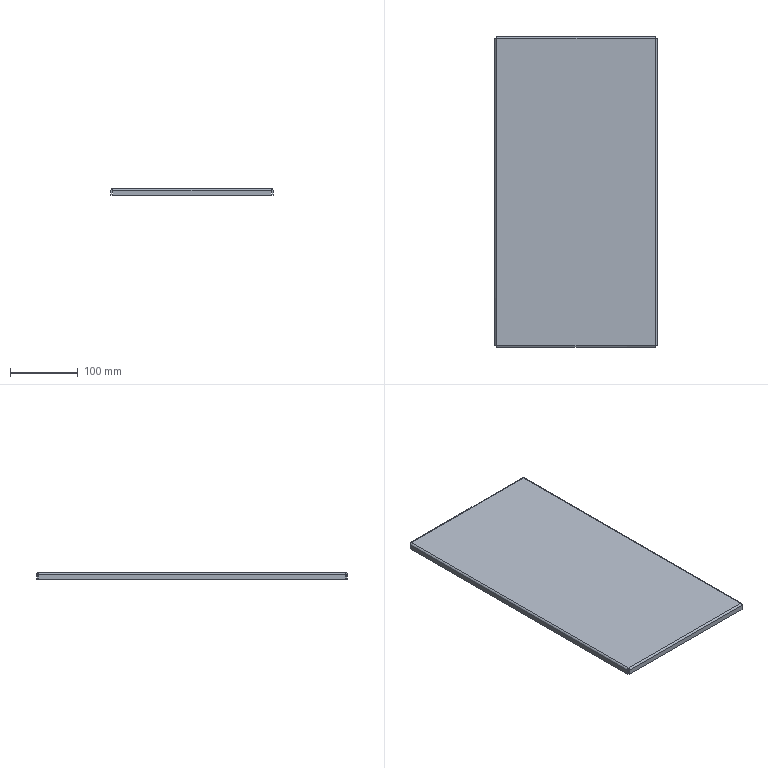Part | STEP file | 11-FG-JX01311 | 1 solid | 38 faces | box 240 x 460 x 10 mm | volume 240740 mm3 | plane 22 | spline 8 | cylinder 8 | commonest cylinder face diameters 1.473 x4 5.473 x4
STEP:
#1=CARTESIAN_POINT('',(117.263,-227.263,-2.));
#2=VERTEX_POINT('',#1);
#3=CARTESIAN_POINT('',(117.263,227.263,-2.));
#4=VERTEX_POINT('',#3);
#5=CARTESIAN_POINT('',(117.263,-227.293,-2.));
#6=DIRECTION('',(0.,1.,0.));
#7=VECTOR('',#6,1000.);
#8=LINE('',#5,#7);
#9=EDGE_CURVE('',#2,#4,#8,.T.);
#10=ORIENTED_EDGE('',*,*,#9,.F.);
#11=CARTESIAN_POINT('',(-117.263,-227.263,-2.));
#12=VERTEX_POINT('',#11);
#13=CARTESIAN_POINT('',(-117.293,-227.263,-2.));
#14=DIRECTION('',(1.,0.,0.));
#15=VECTOR('',#14,1000.);
#16=LINE('',#13,#15);
#17=EDGE_CURVE('',#12,#2,#16,.T.);
#18=ORIENTED_EDGE('',*,*,#17,.F.);
#19=CARTESIAN_POINT('',(-117.263,227.263,-2.));
#20=VERTEX_POINT('',#19);
#21=CARTESIAN_POINT('',(-117.263,227.293,-2.));
#22=DIRECTION('',(0.,-1.,0.));
#23=VECTOR('',#22,1000.);
#24=LINE('',#21,#23);
#25=EDGE_CURVE('',#20,#12,#24,.T.);
#26=ORIENTED_EDGE('',*,*,#25,.F.);
#27=CARTESIAN_POINT('',(117.293,227.263,-2.));
#28=DIRECTION('',(-1.,0.,0.));
#29=VECTOR('',#28,1000.);
#30=LINE('',#27,#29);
#31=EDGE_CURVE('',#4,#20,#30,.T.);
#32=ORIENTED_EDGE('',*,*,#31,.F.);
#33=EDGE_LOOP('',(#10,#18,#26,#32));
#34=FACE_OUTER_BOUND('',#33,.T.);
#35=CARTESIAN_POINT('',(0.,0.,-2.));
#36=DIRECTION('',(0.,0.,1.));
#37=DIRECTION('',(1.,0.,0.));
#38=AXIS2_PLACEMENT_3D('',#35,#36,#37);
#39=PLANE('',#38);
#40=ADVANCED_FACE('',(#34),#39,.F.);
#41=CARTESIAN_POINT('',(-117.263,-227.263,0.));
#42=VERTEX_POINT('',#41);
#43=CARTESIAN_POINT('',(117.263,-227.263,0.));
#44=VERTEX_POINT('',#43);
#45=CARTESIAN_POINT('',(-117.293,-227.263,0.));
#46=DIRECTION('',(1.,0.,0.));
#47=VECTOR('',#46,1000.);
#48=LINE('',#45,#47);
#49=EDGE_CURVE('',#42,#44,#48,.T.);
#50=ORIENTED_EDGE('',*,*,#49,.T.);
#51=CARTESIAN_POINT('',(117.263,227.263,0.));
#52=VERTEX_POINT('',#51);
#53=CARTESIAN_POINT('',(117.263,-227.293,0.));
#54=DIRECTION('',(0.,1.,0.));
#55=VECTOR('',#54,1000.);
#56=LINE('',#53,#55);
#57=EDGE_CURVE('',#44,#52,#56,.T.);
#58=ORIENTED_EDGE('',*,*,#57,.T.);
#59=CARTESIAN_POINT('',(-117.263,227.263,0.));
#60=VERTEX_POINT('',#59);
#61=CARTESIAN_POINT('',(117.293,227.263,0.));
#62=DIRECTION('',(-1.,0.,0.));
#63=VECTOR('',#62,1000.);
#64=LINE('',#61,#63);
#65=EDGE_CURVE('',#52,#60,#64,.T.);
#66=ORIENTED_EDGE('',*,*,#65,.T.);
#67=CARTESIAN_POINT('',(-117.263,227.293,0.));
#68=DIRECTION('',(0.,-1.,0.));
#69=VECTOR('',#68,1000.);
#70=LINE('',#67,#69);
#71=EDGE_CURVE('',#60,#42,#70,.T.);
#72=ORIENTED_EDGE('',*,*,#71,.T.);
#73=EDGE_LOOP('',(#50,#58,#66,#72));
#74=FACE_OUTER_BOUND('',#73,.T.);
#75=CARTESIAN_POINT('',(0.,0.,0.));
#76=DIRECTION('',(0.,0.,1.));
#77=DIRECTION('',(1.,0.,0.));
#78=AXIS2_PLACEMENT_3D('',#75,#76,#77);
#79=PLANE('',#78);
#80=ADVANCED_FACE('',(#74),#79,.T.);
#81=CARTESIAN_POINT('',(-117.293,230.,-2.737));
#82=VERTEX_POINT('',#81);
#83=CARTESIAN_POINT('',(-117.293,228.,-2.737));
#84=VERTEX_POINT('',#83);
#85=CARTESIAN_POINT('',(-117.293,228.,-2.737));
#86=DIRECTION('',(0.,-1.,0.));
#87=VECTOR('',#86,1000.);
#88=LINE('',#85,#87);
#89=EDGE_CURVE('',#82,#84,#88,.T.);
#90=ORIENTED_EDGE('',*,*,#89,.T.);
#91=CARTESIAN_POINT('',(-117.263,227.263,-2.));
#92=CARTESIAN_POINT('',(-117.268,227.456,-2.));
#93=CARTESIAN_POINT('',(-117.273,227.648,-2.079));
#94=CARTESIAN_POINT('',(-117.283,227.921,-2.352));
#95=CARTESIAN_POINT('',(-117.288,228.,-2.544));
#96=CARTESIAN_POINT('',(-117.293,228.,-2.737));
#97=B_SPLINE_CURVE_WITH_KNOTS('',3,(#91,#92,#93,#94,#95,#96),.UNSPECIFIED.,.F.,.F.,(4,2,4),(0.,0.5,1.),.UNSPECIFIED.);
#98=EDGE_CURVE('',#20,#84,#97,.T.);
#99=ORIENTED_EDGE('',*,*,#98,.F.);
#100=CARTESIAN_POINT('',(-117.263,227.263,-2.));
#101=DIRECTION('',(0.,0.,1.));
#102=VECTOR('',#101,1000.);
#103=LINE('',#100,#102);
#104=EDGE_CURVE('',#20,#60,#103,.T.);
#105=ORIENTED_EDGE('',*,*,#104,.T.);
#106=CARTESIAN_POINT('',(-117.263,227.263,0.));
#107=CARTESIAN_POINT('',(-117.266,227.622,0.));
#108=CARTESIAN_POINT('',(-117.268,227.98,-0.07123));
#109=CARTESIAN_POINT('',(-117.273,228.642,-0.3454));
#110=CARTESIAN_POINT('',(-117.276,228.945,-0.5482));
#111=CARTESIAN_POINT('',(-117.281,229.452,-1.055));
#112=CARTESIAN_POINT('',(-117.283,229.655,-1.358));
#113=CARTESIAN_POINT('',(-117.288,229.929,-2.02));
#114=CARTESIAN_POINT('',(-117.29,230.,-2.378));
#115=CARTESIAN_POINT('',(-117.293,230.,-2.737));
#116=B_SPLINE_CURVE_WITH_KNOTS('',3,(#106,#107,#108,#109,#110,#111,#112,#113,#114,#115),.UNSPECIFIED.,.F.,.F.,(4,2,2,2,4),(0.,0.25,0.5,0.75,1.),.UNSPECIFIED.);
#117=EDGE_CURVE('',#60,#82,#116,.T.);
#118=ORIENTED_EDGE('',*,*,#117,.T.);
#119=EDGE_LOOP('',(#90,#99,#105,#118));
#120=FACE_OUTER_BOUND('',#119,.T.);
#121=CARTESIAN_POINT('',(-117.263,227.263,0.02));
#122=CARTESIAN_POINT('',(-117.266,227.624,0.02));
#123=CARTESIAN_POINT('',(-117.268,227.985,-0.05175));
#124=CARTESIAN_POINT('',(-117.273,228.652,-0.3279));
#125=CARTESIAN_POINT('',(-117.276,228.957,-0.5322));
#126=CARTESIAN_POINT('',(-117.281,229.468,-1.043));
#127=CARTESIAN_POINT('',(-117.283,229.672,-1.348));
#128=CARTESIAN_POINT('',(-117.288,229.948,-2.015));
#129=CARTESIAN_POINT('',(-117.29,230.02,-2.376));
#130=CARTESIAN_POINT('',(-117.293,230.02,-2.737));
#131=CARTESIAN_POINT('',(-117.263,227.263,0.));
#132=CARTESIAN_POINT('',(-117.266,227.622,0.));
#133=CARTESIAN_POINT('',(-117.268,227.98,-0.07123));
#134=CARTESIAN_POINT('',(-117.273,228.642,-0.3454));
#135=CARTESIAN_POINT('',(-117.276,228.945,-0.5482));
#136=CARTESIAN_POINT('',(-117.281,229.452,-1.055));
#137=CARTESIAN_POINT('',(-117.283,229.655,-1.358));
#138=CARTESIAN_POINT('',(-117.288,229.929,-2.02));
#139=CARTESIAN_POINT('',(-117.29,230.,-2.378));
#140=CARTESIAN_POINT('',(-117.293,230.,-2.737));
#141=CARTESIAN_POINT('',(-117.263,227.263,-2.));
#142=CARTESIAN_POINT('',(-117.266,227.36,-2.));
#143=CARTESIAN_POINT('',(-117.268,227.456,-2.019));
#144=CARTESIAN_POINT('',(-117.273,227.634,-2.093));
#145=CARTESIAN_POINT('',(-117.276,227.716,-2.148));
#146=CARTESIAN_POINT('',(-117.281,227.852,-2.284));
#147=CARTESIAN_POINT('',(-117.283,227.907,-2.366));
#148=CARTESIAN_POINT('',(-117.288,227.981,-2.544));
#149=CARTESIAN_POINT('',(-117.29,228.,-2.64));
#150=CARTESIAN_POINT('',(-117.293,228.,-2.737));
#151=CARTESIAN_POINT('',(-117.263,227.263,-2.02));
#152=CARTESIAN_POINT('',(-117.266,227.357,-2.02));
#153=CARTESIAN_POINT('',(-117.268,227.451,-2.039));
#154=CARTESIAN_POINT('',(-117.273,227.624,-2.111));
#155=CARTESIAN_POINT('',(-117.276,227.704,-2.164));
#156=CARTESIAN_POINT('',(-117.281,227.836,-2.296));
#157=CARTESIAN_POINT('',(-117.283,227.889,-2.376));
#158=CARTESIAN_POINT('',(-117.288,227.961,-2.549));
#159=CARTESIAN_POINT('',(-117.29,227.98,-2.643));
#160=CARTESIAN_POINT('',(-117.293,227.98,-2.737));
#161=B_SPLINE_SURFACE_WITH_KNOTS('',1,3,((#121,#122,#123,#124,#125,#126,#127,#128,#129,#130),(#131,#132,#133,#134,#135,#136,#137,#138,#139,#140),(#141,#142,#143,#144,#145,#146,#147,#148,#149,#150),(#151,#152,#153,#154,#155,#156,#157,#158,#159,#160)),.UNSPECIFIED.,.F.,.F.,.F.,(2,1,1,2),(4,2,2,2,4),(-0.01,0.,1.,1.01),(0.,0.25,0.5,0.75,1.),.UNSPECIFIED.);
#162=ADVANCED_FACE('',(#120),#161,.F.);
#163=CARTESIAN_POINT('',(117.293,228.,-2.737));
#164=VERTEX_POINT('',#163);
#165=CARTESIAN_POINT('',(117.293,228.,-2.737));
#166=CARTESIAN_POINT('',(117.288,228.,-2.544));
#167=CARTESIAN_POINT('',(117.283,227.921,-2.352));
#168=CARTESIAN_POINT('',(117.273,227.648,-2.079));
#169=CARTESIAN_POINT('',(117.268,227.456,-2.));
#170=CARTESIAN_POINT('',(117.263,227.263,-2.));
#171=B_SPLINE_CURVE_WITH_KNOTS('',3,(#165,#166,#167,#168,#169,#170),.UNSPECIFIED.,.F.,.F.,(4,2,4),(0.,0.5,1.),.UNSPECIFIED.);
#172=EDGE_CURVE('',#164,#4,#171,.T.);
#173=ORIENTED_EDGE('',*,*,#172,.F.);
#174=CARTESIAN_POINT('',(117.293,230.,-2.737));
#175=VERTEX_POINT('',#174);
#176=CARTESIAN_POINT('',(117.293,228.,-2.737));
#177=DIRECTION('',(0.,-1.,0.));
#178=VECTOR('',#177,1000.);
#179=LINE('',#176,#178);
#180=EDGE_CURVE('',#175,#164,#179,.T.);
#181=ORIENTED_EDGE('',*,*,#180,.F.);
#182=CARTESIAN_POINT('',(117.293,230.,-2.737));
#183=CARTESIAN_POINT('',(117.29,230.,-2.378));
#184=CARTESIAN_POINT('',(117.288,229.929,-2.02));
#185=CARTESIAN_POINT('',(117.283,229.655,-1.358));
#186=CARTESIAN_POINT('',(117.281,229.452,-1.055));
#187=CARTESIAN_POINT('',(117.276,228.945,-0.5482));
#188=CARTESIAN_POINT('',(117.273,228.642,-0.3454));
#189=CARTESIAN_POINT('',(117.268,227.98,-0.07123));
#190=CARTESIAN_POINT('',(117.266,227.622,0.));
#191=CARTESIAN_POINT('',(117.263,227.263,0.));
#192=B_SPLINE_CURVE_WITH_KNOTS('',3,(#182,#183,#184,#185,#186,#187,#188,#189,#190,#191),.UNSPECIFIED.,.F.,.F.,(4,2,2,2,4),(0.,0.25,0.5,0.75,1.),.UNSPECIFIED.);
#193=EDGE_CURVE('',#175,#52,#192,.T.);
#194=ORIENTED_EDGE('',*,*,#193,.T.);
#195=CARTESIAN_POINT('',(117.263,227.263,-2.));
#196=DIRECTION('',(0.,0.,1.));
#197=VECTOR('',#196,1000.);
#198=LINE('',#195,#197);
#199=EDGE_CURVE('',#4,#52,#198,.T.);
#200=ORIENTED_EDGE('',*,*,#199,.F.);
#201=EDGE_LOOP('',(#173,#181,#194,#200));
#202=FACE_OUTER_BOUND('',#201,.T.);
#203=CARTESIAN_POINT('',(117.293,230.02,-2.737));
#204=CARTESIAN_POINT('',(117.29,230.02,-2.376));
#205=CARTESIAN_POINT('',(117.288,229.948,-2.015));
#206=CARTESIAN_POINT('',(117.283,229.672,-1.348));
#207=CARTESIAN_POINT('',(117.281,229.468,-1.043));
#208=CARTESIAN_POINT('',(117.276,228.957,-0.5322));
#209=CARTESIAN_POINT('',(117.273,228.652,-0.3279));
#210=CARTESIAN_POINT('',(117.268,227.985,-0.05175));
#211=CARTESIAN_POINT('',(117.266,227.624,0.02));
#212=CARTESIAN_POINT('',(117.263,227.263,0.02));
#213=CARTESIAN_POINT('',(117.293,230.,-2.737));
#214=CARTESIAN_POINT('',(117.29,230.,-2.378));
#215=CARTESIAN_POINT('',(117.288,229.929,-2.02));
#216=CARTESIAN_POINT('',(117.283,229.655,-1.358));
#217=CARTESIAN_POINT('',(117.281,229.452,-1.055));
#218=CARTESIAN_POINT('',(117.276,228.945,-0.5482));
#219=CARTESIAN_POINT('',(117.273,228.642,-0.3454));
#220=CARTESIAN_POINT('',(117.268,227.98,-0.07123));
#221=CARTESIAN_POINT('',(117.266,227.622,0.));
#222=CARTESIAN_POINT('',(117.263,227.263,0.));
#223=CARTESIAN_POINT('',(117.293,228.,-2.737));
#224=CARTESIAN_POINT('',(117.29,228.,-2.64));
#225=CARTESIAN_POINT('',(117.288,227.981,-2.544));
#226=CARTESIAN_POINT('',(117.283,227.907,-2.366));
#227=CARTESIAN_POINT('',(117.281,227.852,-2.284));
#228=CARTESIAN_POINT('',(117.276,227.716,-2.148));
#229=CARTESIAN_POINT('',(117.273,227.634,-2.093));
#230=CARTESIAN_POINT('',(117.268,227.456,-2.019));
#231=CARTESIAN_POINT('',(117.266,227.36,-2.));
#232=CARTESIAN_POINT('',(117.263,227.263,-2.));
#233=CARTESIAN_POINT('',(117.293,227.98,-2.737));
#234=CARTESIAN_POINT('',(117.29,227.98,-2.643));
#235=CARTESIAN_POINT('',(117.288,227.961,-2.549));
#236=CARTESIAN_POINT('',(117.283,227.889,-2.376));
#237=CARTESIAN_POINT('',(117.281,227.836,-2.296));
#238=CARTESIAN_POINT('',(117.276,227.704,-2.164));
#239=CARTESIAN_POINT('',(117.273,227.624,-2.111));
#240=CARTESIAN_POINT('',(117.268,227.451,-2.039));
#241=CARTESIAN_POINT('',(117.266,227.357,-2.02));
#242=CARTESIAN_POINT('',(117.263,227.263,-2.02));
#243=B_SPLINE_SURFACE_WITH_KNOTS('',1,3,((#203,#204,#205,#206,#207,#208,#209,#210,#211,#212),(#213,#214,#215,#216,#217,#218,#219,#220,#221,#222),(#223,#224,#225,#226,#227,#228,#229,#230,#231,#232),(#233,#234,#235,#236,#237,#238,#239,#240,#241,#242)),.UNSPECIFIED.,.F.,.F.,.F.,(2,1,1,2),(4,2,2,2,4),(-0.01,0.,1.,1.01),(0.,0.25,0.5,0.75,1.),.UNSPECIFIED.);
#244=ADVANCED_FACE('',(#202),#243,.F.);
#245=ORIENTED_EDGE('',*,*,#65,.F.);
#246=ORIENTED_EDGE('',*,*,#193,.F.);
#247=CARTESIAN_POINT('',(0.,230.,-2.737));
#248=DIRECTION('',(1.,0.,0.));
#249=VECTOR('',#248,1000.);
#250=LINE('',#247,#249);
#251=EDGE_CURVE('',#82,#175,#250,.T.);
#252=ORIENTED_EDGE('',*,*,#251,.F.);
#253=ORIENTED_EDGE('',*,*,#117,.F.);
#254=EDGE_LOOP('',(#245,#246,#252,#253));
#255=FACE_OUTER_BOUND('',#254,.T.);
#256=CARTESIAN_POINT('',(117.293,227.263,-2.737));
#257=DIRECTION('',(1.,0.,0.));
#258=DIRECTION('',(0.,1.,0.));
#259=AXIS2_PLACEMENT_3D('',#256,#257,#258);
#260=CYLINDRICAL_SURFACE('',#259,2.737);
#261=ADVANCED_FACE('',(#255),#260,.T.);
#262=ORIENTED_EDGE('',*,*,#31,.T.);
#263=ORIENTED_EDGE('',*,*,#98,.T.);
#264=CARTESIAN_POINT('',(-120.,228.,-2.737));
#265=DIRECTION('',(1.,0.,0.));
#266=VECTOR('',#265,1000.);
#267=LINE('',#264,#266);
#268=EDGE_CURVE('',#84,#164,#267,.T.);
#269=ORIENTED_EDGE('',*,*,#268,.T.);
#270=ORIENTED_EDGE('',*,*,#172,.T.);
#271=EDGE_LOOP('',(#262,#263,#269,#270));
#272=FACE_OUTER_BOUND('',#271,.T.);
#273=CARTESIAN_POINT('',(117.293,227.263,-2.737));
#274=DIRECTION('',(1.,0.,0.));
#275=DIRECTION('',(0.,1.,0.));
#276=AXIS2_PLACEMENT_3D('',#273,#274,#275);
#277=CYLINDRICAL_SURFACE('',#276,0.7366);
#278=ADVANCED_FACE('',(#272),#277,.F.);
#279=CARTESIAN_POINT('',(-117.293,228.,-10.));
#280=VERTEX_POINT('',#279);
#281=CARTESIAN_POINT('',(-117.293,230.,-10.));
#282=VERTEX_POINT('',#281);
#283=CARTESIAN_POINT('',(-117.293,230.,-10.));
#284=DIRECTION('',(0.,1.,0.));
#285=VECTOR('',#284,1000.);
#286=LINE('',#283,#285);
#287=EDGE_CURVE('',#280,#282,#286,.T.);
#288=ORIENTED_EDGE('',*,*,#287,.F.);
#289=CARTESIAN_POINT('',(-117.293,228.,0.));
#290=DIRECTION('',(0.,0.,-1.));
#291=VECTOR('',#290,1000.);
#292=LINE('',#289,#291);
#293=EDGE_CURVE('',#84,#280,#292,.T.);
#294=ORIENTED_EDGE('',*,*,#293,.F.);
#295=ORIENTED_EDGE('',*,*,#89,.F.);
#296=CARTESIAN_POINT('',(-117.293,230.,0.));
#297=DIRECTION('',(0.,0.,1.));
#298=VECTOR('',#297,1000.);
#299=LINE('',#296,#298);
#300=EDGE_CURVE('',#282,#82,#299,.T.);
#301=ORIENTED_EDGE('',*,*,#300,.F.);
#302=EDGE_LOOP('',(#288,#294,#295,#301));
#303=FACE_OUTER_BOUND('',#302,.T.);
#304=CARTESIAN_POINT('',(-117.293,228.,-2.));
#305=DIRECTION('',(-1.,0.,0.));
#306=DIRECTION('',(0.,0.,1.));
#307=AXIS2_PLACEMENT_3D('',#304,#305,#306);
#308=PLANE('',#307);
#309=ADVANCED_FACE('',(#303),#308,.T.);
#310=CARTESIAN_POINT('',(117.293,230.,-10.));
#311=VERTEX_POINT('',#310);
#312=CARTESIAN_POINT('',(117.293,230.,-2.));
#313=DIRECTION('',(0.,0.,1.));
#314=VECTOR('',#313,1000.);
#315=LINE('',#312,#314);
#316=EDGE_CURVE('',#311,#175,#315,.T.);
#317=ORIENTED_EDGE('',*,*,#316,.F.);
#318=CARTESIAN_POINT('',(120.,230.,-10.));
#319=DIRECTION('',(1.,0.,0.));
#320=VECTOR('',#319,1000.);
#321=LINE('',#318,#320);
#322=EDGE_CURVE('',#282,#311,#321,.T.);
#323=ORIENTED_EDGE('',*,*,#322,.F.);
#324=ORIENTED_EDGE('',*,*,#300,.T.);
#325=ORIENTED_EDGE('',*,*,#251,.T.);
#326=EDGE_LOOP('',(#317,#323,#324,#325));
#327=FACE_OUTER_BOUND('',#326,.T.);
#328=CARTESIAN_POINT('',(0.,230.,0.));
#329=DIRECTION('',(0.,1.,0.));
#330=DIRECTION('',(0.,0.,1.));
#331=AXIS2_PLACEMENT_3D('',#328,#329,#330);
#332=PLANE('',#331);
#333=ADVANCED_FACE('',(#327),#332,.T.);
#334=CARTESIAN_POINT('',(117.293,228.,-10.));
#335=VERTEX_POINT('',#334);
#336=CARTESIAN_POINT('',(0.,228.,-10.));
#337=DIRECTION('',(1.,0.,0.));
#338=VECTOR('',#337,1000.);
#339=LINE('',#336,#338);
#340=EDGE_CURVE('',#280,#335,#339,.T.);
#341=ORIENTED_EDGE('',*,*,#340,.T.);
#342=CARTESIAN_POINT('',(117.293,228.,-2.));
#343=DIRECTION('',(0.,0.,-1.));
#344=VECTOR('',#343,1000.);
#345=LINE('',#342,#344);
#346=EDGE_CURVE('',#164,#335,#345,.T.);
#347=ORIENTED_EDGE('',*,*,#346,.F.);
#348=ORIENTED_EDGE('',*,*,#268,.F.);
#349=ORIENTED_EDGE('',*,*,#293,.T.);
#350=EDGE_LOOP('',(#341,#347,#348,#349));
#351=FACE_OUTER_BOUND('',#350,.T.);
#352=CARTESIAN_POINT('',(0.,228.,0.));
#353=DIRECTION('',(0.,1.,0.));
#354=DIRECTION('',(0.,0.,1.));
#355=AXIS2_PLACEMENT_3D('',#352,#353,#354);
#356=PLANE('',#355);
#357=ADVANCED_FACE('',(#351),#356,.F.);
#358=CARTESIAN_POINT('',(117.293,228.,-10.));
#359=DIRECTION('',(0.,1.,0.));
#360=VECTOR('',#359,1000.);
#361=LINE('',#358,#360);
#362=EDGE_CURVE('',#335,#311,#361,.T.);
#363=ORIENTED_EDGE('',*,*,#362,.F.);
#364=ORIENTED_EDGE('',*,*,#340,.F.);
#365=ORIENTED_EDGE('',*,*,#287,.T.);
#366=ORIENTED_EDGE('',*,*,#322,.T.);
#367=EDGE_LOOP('',(#363,#364,#365,#366));
#368=FACE_OUTER_BOUND('',#367,.T.);
#369=CARTESIAN_POINT('',(120.,230.,-10.));
#370=DIRECTION('',(0.,0.,-1.));
#371=DIRECTION('',(0.,1.,0.));
#372=AXIS2_PLACEMENT_3D('',#369,#370,#371);
#373=PLANE('',#372);
#374=ADVANCED_FACE('',(#368),#373,.T.);
#375=ORIENTED_EDGE('',*,*,#346,.T.);
#376=ORIENTED_EDGE('',*,*,#362,.T.);
#377=ORIENTED_EDGE('',*,*,#316,.T.);
#378=ORIENTED_EDGE('',*,*,#180,.T.);
#379=EDGE_LOOP('',(#375,#376,#377,#378));
#380=FACE_OUTER_BOUND('',#379,.T.);
#381=CARTESIAN_POINT('',(117.293,228.,-2.));
#382=DIRECTION('',(-1.,0.,0.));
#383=DIRECTION('',(0.,0.,1.));
#384=AXIS2_PLACEMENT_3D('',#381,#382,#383);
#385=PLANE('',#384);
#386=ADVANCED_FACE('',(#380),#385,.F.);
#387=CARTESIAN_POINT('',(-120.,-227.293,-2.737));
#388=VERTEX_POINT('',#387);
#389=CARTESIAN_POINT('',(-118.,-227.293,-2.737));
#390=VERTEX_POINT('',#389);
#391=CARTESIAN_POINT('',(-118.,-227.293,-2.737));
#392=DIRECTION('',(1.,0.,0.));
#393=VECTOR('',#392,1000.);
#394=LINE('',#391,#393);
#395=EDGE_CURVE('',#388,#390,#394,.T.);
#396=ORIENTED_EDGE('',*,*,#395,.T.);
#397=CARTESIAN_POINT('',(-117.263,-227.263,-2.));
#398=CARTESIAN_POINT('',(-117.456,-227.268,-2.));
#399=CARTESIAN_POINT('',(-117.648,-227.273,-2.079));
#400=CARTESIAN_POINT('',(-117.921,-227.283,-2.352));
#401=CARTESIAN_POINT('',(-118.,-227.288,-2.544));
#402=CARTESIAN_POINT('',(-118.,-227.293,-2.737));
#403=B_SPLINE_CURVE_WITH_KNOTS('',3,(#397,#398,#399,#400,#401,#402),.UNSPECIFIED.,.F.,.F.,(4,2,4),(0.,0.5,1.),.UNSPECIFIED.);
#404=EDGE_CURVE('',#12,#390,#403,.T.);
#405=ORIENTED_EDGE('',*,*,#404,.F.);
#406=CARTESIAN_POINT('',(-117.263,-227.263,-2.));
#407=DIRECTION('',(0.,0.,1.));
#408=VECTOR('',#407,1000.);
#409=LINE('',#406,#408);
#410=EDGE_CURVE('',#12,#42,#409,.T.);
#411=ORIENTED_EDGE('',*,*,#410,.T.);
#412=CARTESIAN_POINT('',(-117.263,-227.263,0.));
#413=CARTESIAN_POINT('',(-117.622,-227.266,0.));
#414=CARTESIAN_POINT('',(-117.98,-227.268,-0.07123));
#415=CARTESIAN_POINT('',(-118.642,-227.273,-0.3454));
#416=CARTESIAN_POINT('',(-118.945,-227.276,-0.5482));
#417=CARTESIAN_POINT('',(-119.452,-227.281,-1.055));
#418=CARTESIAN_POINT('',(-119.655,-227.283,-1.358));
#419=CARTESIAN_POINT('',(-119.929,-227.288,-2.02));
#420=CARTESIAN_POINT('',(-120.,-227.29,-2.378));
#421=CARTESIAN_POINT('',(-120.,-227.293,-2.737));
#422=B_SPLINE_CURVE_WITH_KNOTS('',3,(#412,#413,#414,#415,#416,#417,#418,#419,#420,#421),.UNSPECIFIED.,.F.,.F.,(4,2,2,2,4),(0.,0.25,0.5,0.75,1.),.UNSPECIFIED.);
#423=EDGE_CURVE('',#42,#388,#422,.T.);
#424=ORIENTED_EDGE('',*,*,#423,.T.);
#425=EDGE_LOOP('',(#396,#405,#411,#424));
#426=FACE_OUTER_BOUND('',#425,.T.);
#427=CARTESIAN_POINT('',(-117.263,-227.263,0.02));
#428=CARTESIAN_POINT('',(-117.624,-227.266,0.02));
#429=CARTESIAN_POINT('',(-117.985,-227.268,-0.05175));
#430=CARTESIAN_POINT('',(-118.652,-227.273,-0.3279));
#431=CARTESIAN_POINT('',(-118.957,-227.276,-0.5322));
#432=CARTESIAN_POINT('',(-119.468,-227.281,-1.043));
#433=CARTESIAN_POINT('',(-119.672,-227.283,-1.348));
#434=CARTESIAN_POINT('',(-119.948,-227.288,-2.015));
#435=CARTESIAN_POINT('',(-120.02,-227.29,-2.376));
#436=CARTESIAN_POINT('',(-120.02,-227.293,-2.737));
#437=CARTESIAN_POINT('',(-117.263,-227.263,0.));
#438=CARTESIAN_POINT('',(-117.622,-227.266,0.));
#439=CARTESIAN_POINT('',(-117.98,-227.268,-0.07123));
#440=CARTESIAN_POINT('',(-118.642,-227.273,-0.3454));
#441=CARTESIAN_POINT('',(-118.945,-227.276,-0.5482));
#442=CARTESIAN_POINT('',(-119.452,-227.281,-1.055));
#443=CARTESIAN_POINT('',(-119.655,-227.283,-1.358));
#444=CARTESIAN_POINT('',(-119.929,-227.288,-2.02));
#445=CARTESIAN_POINT('',(-120.,-227.29,-2.378));
#446=CARTESIAN_POINT('',(-120.,-227.293,-2.737));
#447=CARTESIAN_POINT('',(-117.263,-227.263,-2.));
#448=CARTESIAN_POINT('',(-117.36,-227.266,-2.));
#449=CARTESIAN_POINT('',(-117.456,-227.268,-2.019));
#450=CARTESIAN_POINT('',(-117.634,-227.273,-2.093));
#451=CARTESIAN_POINT('',(-117.716,-227.276,-2.148));
#452=CARTESIAN_POINT('',(-117.852,-227.281,-2.284));
#453=CARTESIAN_POINT('',(-117.907,-227.283,-2.366));
#454=CARTESIAN_POINT('',(-117.981,-227.288,-2.544));
#455=CARTESIAN_POINT('',(-118.,-227.29,-2.64));
#456=CARTESIAN_POINT('',(-118.,-227.293,-2.737));
#457=CARTESIAN_POINT('',(-117.263,-227.263,-2.02));
#458=CARTESIAN_POINT('',(-117.357,-227.266,-2.02));
#459=CARTESIAN_POINT('',(-117.451,-227.268,-2.039));
#460=CARTESIAN_POINT('',(-117.624,-227.273,-2.111));
#461=CARTESIAN_POINT('',(-117.704,-227.276,-2.164));
#462=CARTESIAN_POINT('',(-117.836,-227.281,-2.296));
#463=CARTESIAN_POINT('',(-117.889,-227.283,-2.376));
#464=CARTESIAN_POINT('',(-117.961,-227.288,-2.549));
#465=CARTESIAN_POINT('',(-117.98,-227.29,-2.643));
#466=CARTESIAN_POINT('',(-117.98,-227.293,-2.737));
#467=B_SPLINE_SURFACE_WITH_KNOTS('',1,3,((#427,#428,#429,#430,#431,#432,#433,#434,#435,#436),(#437,#438,#439,#440,#441,#442,#443,#444,#445,#446),(#447,#448,#449,#450,#451,#452,#453,#454,#455,#456),(#457,#458,#459,#460,#461,#462,#463,#464,#465,#466)),.UNSPECIFIED.,.F.,.F.,.F.,(2,1,1,2),(4,2,2,2,4),(-0.01,0.,1.,1.01),(0.,0.25,0.5,0.75,1.),.UNSPECIFIED.);
#468=ADVANCED_FACE('',(#426),#467,.F.);
#469=CARTESIAN_POINT('',(-118.,227.293,-2.737));
#470=VERTEX_POINT('',#469);
#471=CARTESIAN_POINT('',(-118.,227.293,-2.737));
#472=CARTESIAN_POINT('',(-118.,227.288,-2.544));
#473=CARTESIAN_POINT('',(-117.921,227.283,-2.352));
#474=CARTESIAN_POINT('',(-117.648,227.273,-2.079));
#475=CARTESIAN_POINT('',(-117.456,227.268,-2.));
#476=CARTESIAN_POINT('',(-117.263,227.263,-2.));
#477=B_SPLINE_CURVE_WITH_KNOTS('',3,(#471,#472,#473,#474,#475,#476),.UNSPECIFIED.,.F.,.F.,(4,2,4),(0.,0.5,1.),.UNSPECIFIED.);
#478=EDGE_CURVE('',#470,#20,#477,.T.);
#479=ORIENTED_EDGE('',*,*,#478,.F.);
#480=CARTESIAN_POINT('',(-120.,227.293,-2.737));
#481=VERTEX_POINT('',#480);
#482=CARTESIAN_POINT('',(-118.,227.293,-2.737));
#483=DIRECTION('',(1.,0.,0.));
#484=VECTOR('',#483,1000.);
#485=LINE('',#482,#484);
#486=EDGE_CURVE('',#481,#470,#485,.T.);
#487=ORIENTED_EDGE('',*,*,#486,.F.);
#488=CARTESIAN_POINT('',(-120.,227.293,-2.737));
#489=CARTESIAN_POINT('',(-120.,227.29,-2.378));
#490=CARTESIAN_POINT('',(-119.929,227.288,-2.02));
#491=CARTESIAN_POINT('',(-119.655,227.283,-1.358));
#492=CARTESIAN_POINT('',(-119.452,227.281,-1.055));
#493=CARTESIAN_POINT('',(-118.945,227.276,-0.5482));
#494=CARTESIAN_POINT('',(-118.642,227.273,-0.3454));
#495=CARTESIAN_POINT('',(-117.98,227.268,-0.07123));
#496=CARTESIAN_POINT('',(-117.622,227.266,0.));
#497=CARTESIAN_POINT('',(-117.263,227.263,0.));
#498=B_SPLINE_CURVE_WITH_KNOTS('',3,(#488,#489,#490,#491,#492,#493,#494,#495,#496,#497),.UNSPECIFIED.,.F.,.F.,(4,2,2,2,4),(0.,0.25,0.5,0.75,1.),.UNSPECIFIED.);
#499=EDGE_CURVE('',#481,#60,#498,.T.);
#500=ORIENTED_EDGE('',*,*,#499,.T.);
#501=ORIENTED_EDGE('',*,*,#104,.F.);
#502=EDGE_LOOP('',(#479,#487,#500,#501));
#503=FACE_OUTER_BOUND('',#502,.T.);
#504=CARTESIAN_POINT('',(-120.02,227.293,-2.737));
#505=CARTESIAN_POINT('',(-120.02,227.29,-2.376));
#506=CARTESIAN_POINT('',(-119.948,227.288,-2.015));
#507=CARTESIAN_POINT('',(-119.672,227.283,-1.348));
#508=CARTESIAN_POINT('',(-119.468,227.281,-1.043));
#509=CARTESIAN_POINT('',(-118.957,227.276,-0.5322));
#510=CARTESIAN_POINT('',(-118.652,227.273,-0.3279));
#511=CARTESIAN_POINT('',(-117.985,227.268,-0.05175));
#512=CARTESIAN_POINT('',(-117.624,227.266,0.02));
#513=CARTESIAN_POINT('',(-117.263,227.263,0.02));
#514=CARTESIAN_POINT('',(-120.,227.293,-2.737));
#515=CARTESIAN_POINT('',(-120.,227.29,-2.378));
#516=CARTESIAN_POINT('',(-119.929,227.288,-2.02));
#517=CARTESIAN_POINT('',(-119.655,227.283,-1.358));
#518=CARTESIAN_POINT('',(-119.452,227.281,-1.055));
#519=CARTESIAN_POINT('',(-118.945,227.276,-0.5482));
#520=CARTESIAN_POINT('',(-118.642,227.273,-0.3454));
#521=CARTESIAN_POINT('',(-117.98,227.268,-0.07123));
#522=CARTESIAN_POINT('',(-117.622,227.266,0.));
#523=CARTESIAN_POINT('',(-117.263,227.263,0.));
#524=CARTESIAN_POINT('',(-118.,227.293,-2.737));
#525=CARTESIAN_POINT('',(-118.,227.29,-2.64));
#526=CARTESIAN_POINT('',(-117.981,227.288,-2.544));
#527=CARTESIAN_POINT('',(-117.907,227.283,-2.366));
#528=CARTESIAN_POINT('',(-117.852,227.281,-2.284));
#529=CARTESIAN_POINT('',(-117.716,227.276,-2.148));
#530=CARTESIAN_POINT('',(-117.634,227.273,-2.093));
#531=CARTESIAN_POINT('',(-117.456,227.268,-2.019));
#532=CARTESIAN_POINT('',(-117.36,227.266,-2.));
#533=CARTESIAN_POINT('',(-117.263,227.263,-2.));
#534=CARTESIAN_POINT('',(-117.98,227.293,-2.737));
#535=CARTESIAN_POINT('',(-117.98,227.29,-2.643));
#536=CARTESIAN_POINT('',(-117.961,227.288,-2.549));
#537=CARTESIAN_POINT('',(-117.889,227.283,-2.376));
#538=CARTESIAN_POINT('',(-117.836,227.281,-2.296));
#539=CARTESIAN_POINT('',(-117.704,227.276,-2.164));
#540=CARTESIAN_POINT('',(-117.624,227.273,-2.111));
#541=CARTESIAN_POINT('',(-117.451,227.268,-2.039));
#542=CARTESIAN_POINT('',(-117.357,227.266,-2.02));
#543=CARTESIAN_POINT('',(-117.263,227.263,-2.02));
#544=B_SPLINE_SURFACE_WITH_KNOTS('',1,3,((#504,#505,#506,#507,#508,#509,#510,#511,#512,#513),(#514,#515,#516,#517,#518,#519,#520,#521,#522,#523),(#524,#525,#526,#527,#528,#529,#530,#531,#532,#533),(#534,#535,#536,#537,#538,#539,#540,#541,#542,#543)),.UNSPECIFIED.,.F.,.F.,.F.,(2,1,1,2),(4,2,2,2,4),(-0.01,0.,1.,1.01),(0.,0.25,0.5,0.75,1.),.UNSPECIFIED.);
#545=ADVANCED_FACE('',(#503),#544,.F.);
#546=ORIENTED_EDGE('',*,*,#71,.F.);
#547=ORIENTED_EDGE('',*,*,#499,.F.);
#548=CARTESIAN_POINT('',(-120.,-230.,-2.737));
#549=DIRECTION('',(0.,-1.,0.));
#550=VECTOR('',#549,1000.);
#551=LINE('',#548,#550);
#552=EDGE_CURVE('',#481,#388,#551,.T.);
#553=ORIENTED_EDGE('',*,*,#552,.T.);
#554=ORIENTED_EDGE('',*,*,#423,.F.);
#555=EDGE_LOOP('',(#546,#547,#553,#554));
#556=FACE_OUTER_BOUND('',#555,.T.);
#557=CARTESIAN_POINT('',(-117.263,227.293,-2.737));
#558=DIRECTION('',(0.,1.,0.));
#559=DIRECTION('',(-1.,0.,0.));
#560=AXIS2_PLACEMENT_3D('',#557,#558,#559);
#561=CYLINDRICAL_SURFACE('',#560,2.737);
#562=ADVANCED_FACE('',(#556),#561,.T.);
#563=ORIENTED_EDGE('',*,*,#25,.T.);
#564=ORIENTED_EDGE('',*,*,#404,.T.);
#565=CARTESIAN_POINT('',(-118.,-230.,-2.737));
#566=DIRECTION('',(0.,1.,0.));
#567=VECTOR('',#566,1000.);
#568=LINE('',#565,#567);
#569=EDGE_CURVE('',#390,#470,#568,.T.);
#570=ORIENTED_EDGE('',*,*,#569,.T.);
#571=ORIENTED_EDGE('',*,*,#478,.T.);
#572=EDGE_LOOP('',(#563,#564,#570,#571));
#573=FACE_OUTER_BOUND('',#572,.T.);
#574=CARTESIAN_POINT('',(-117.263,227.293,-2.737));
#575=DIRECTION('',(0.,1.,0.));
#576=DIRECTION('',(-1.,0.,0.));
#577=AXIS2_PLACEMENT_3D('',#574,#575,#576);
#578=CYLINDRICAL_SURFACE('',#577,0.7366);
#579=ADVANCED_FACE('',(#573),#578,.F.);
#580=CARTESIAN_POINT('',(-118.,-227.293,-10.));
#581=VERTEX_POINT('',#580);
#582=CARTESIAN_POINT('',(-120.,-227.293,-10.));
#583=VERTEX_POINT('',#582);
#584=CARTESIAN_POINT('',(-120.,-227.293,-10.));
#585=DIRECTION('',(-1.,0.,0.));
#586=VECTOR('',#585,1000.);
#587=LINE('',#584,#586);
#588=EDGE_CURVE('',#581,#583,#587,.T.);
#589=ORIENTED_EDGE('',*,*,#588,.F.);
#590=CARTESIAN_POINT('',(-118.,-227.293,0.));
#591=DIRECTION('',(0.,0.,-1.));
#592=VECTOR('',#591,1000.);
#593=LINE('',#590,#592);
#594=EDGE_CURVE('',#390,#581,#593,.T.);
#595=ORIENTED_EDGE('',*,*,#594,.F.);
#596=ORIENTED_EDGE('',*,*,#395,.F.);
#597=CARTESIAN_POINT('',(-120.,-227.293,-2.));
#598=DIRECTION('',(0.,0.,-1.));
#599=VECTOR('',#598,1000.);
#600=LINE('',#597,#599);
#601=EDGE_CURVE('',#388,#583,#600,.T.);
#602=ORIENTED_EDGE('',*,*,#601,.T.);
#603=EDGE_LOOP('',(#589,#595,#596,#602));
#604=FACE_OUTER_BOUND('',#603,.T.);
#605=CARTESIAN_POINT('',(-118.,-227.293,-2.));
#606=DIRECTION('',(0.,-1.,0.));
#607=DIRECTION('',(0.,0.,-1.));
#608=AXIS2_PLACEMENT_3D('',#605,#606,#607);
#609=PLANE('',#608);
#610=ADVANCED_FACE('',(#604),#609,.T.);
#611=ORIENTED_EDGE('',*,*,#552,.F.);
#612=CARTESIAN_POINT('',(-120.,227.293,-10.));
#613=VERTEX_POINT('',#612);
#614=CARTESIAN_POINT('',(-120.,227.293,0.));
#615=DIRECTION('',(0.,0.,-1.));
#616=VECTOR('',#615,1000.);
#617=LINE('',#614,#616);
#618=EDGE_CURVE('',#481,#613,#617,.T.);
#619=ORIENTED_EDGE('',*,*,#618,.T.);
#620=CARTESIAN_POINT('',(-120.,-230.,-10.));
#621=DIRECTION('',(0.,1.,0.));
#622=VECTOR('',#621,1000.);
#623=LINE('',#620,#622);
#624=EDGE_CURVE('',#583,#613,#623,.T.);
#625=ORIENTED_EDGE('',*,*,#624,.F.);
#626=ORIENTED_EDGE('',*,*,#601,.F.);
#627=EDGE_LOOP('',(#611,#619,#625,#626));
#628=FACE_OUTER_BOUND('',#627,.T.);
#629=CARTESIAN_POINT('',(-120.,0.,0.));
#630=DIRECTION('',(1.,0.,0.));
#631=DIRECTION('',(0.,0.,-1.));
#632=AXIS2_PLACEMENT_3D('',#629,#630,#631);
#633=PLANE('',#632);
#634=ADVANCED_FACE('',(#628),#633,.F.);
#635=CARTESIAN_POINT('',(-118.,227.293,-10.));
#636=VERTEX_POINT('',#635);
#637=CARTESIAN_POINT('',(-118.,227.293,-2.));
#638=DIRECTION('',(0.,0.,-1.));
#639=VECTOR('',#638,1000.);
#640=LINE('',#637,#639);
#641=EDGE_CURVE('',#470,#636,#640,.T.);
#642=ORIENTED_EDGE('',*,*,#641,.F.);
#643=ORIENTED_EDGE('',*,*,#569,.F.);
#644=ORIENTED_EDGE('',*,*,#594,.T.);
#645=CARTESIAN_POINT('',(-118.,0.,-10.));
#646=DIRECTION('',(0.,1.,0.));
#647=VECTOR('',#646,1000.);
#648=LINE('',#645,#647);
#649=EDGE_CURVE('',#581,#636,#648,.T.);
#650=ORIENTED_EDGE('',*,*,#649,.T.);
#651=EDGE_LOOP('',(#642,#643,#644,#650));
#652=FACE_OUTER_BOUND('',#651,.T.);
#653=CARTESIAN_POINT('',(-118.,0.,0.));
#654=DIRECTION('',(1.,0.,0.));
#655=DIRECTION('',(0.,0.,-1.));
#656=AXIS2_PLACEMENT_3D('',#653,#654,#655);
#657=PLANE('',#656);
#658=ADVANCED_FACE('',(#652),#657,.T.);
#659=CARTESIAN_POINT('',(-118.,227.293,-10.));
#660=DIRECTION('',(-1.,0.,0.));
#661=VECTOR('',#660,1000.);
#662=LINE('',#659,#661);
#663=EDGE_CURVE('',#636,#613,#662,.T.);
#664=ORIENTED_EDGE('',*,*,#663,.F.);
#665=ORIENTED_EDGE('',*,*,#649,.F.);
#666=ORIENTED_EDGE('',*,*,#588,.T.);
#667=ORIENTED_EDGE('',*,*,#624,.T.);
#668=EDGE_LOOP('',(#664,#665,#666,#667));
#669=FACE_OUTER_BOUND('',#668,.T.);
#670=CARTESIAN_POINT('',(-120.,-230.,-10.));
#671=DIRECTION('',(0.,0.,-1.));
#672=DIRECTION('',(-1.,0.,0.));
#673=AXIS2_PLACEMENT_3D('',#670,#671,#672);
#674=PLANE('',#673);
#675=ADVANCED_FACE('',(#669),#674,.T.);
#676=ORIENTED_EDGE('',*,*,#641,.T.);
#677=ORIENTED_EDGE('',*,*,#663,.T.);
#678=ORIENTED_EDGE('',*,*,#618,.F.);
#679=ORIENTED_EDGE('',*,*,#486,.T.);
#680=EDGE_LOOP('',(#676,#677,#678,#679));
#681=FACE_OUTER_BOUND('',#680,.T.);
#682=CARTESIAN_POINT('',(-118.,227.293,-2.));
#683=DIRECTION('',(0.,-1.,0.));
#684=DIRECTION('',(0.,0.,-1.));
#685=AXIS2_PLACEMENT_3D('',#682,#683,#684);
#686=PLANE('',#685);
#687=ADVANCED_FACE('',(#681),#686,.F.);
#688=CARTESIAN_POINT('',(117.293,-230.,-2.737));
#689=VERTEX_POINT('',#688);
#690=CARTESIAN_POINT('',(117.293,-228.,-2.737));
#691=VERTEX_POINT('',#690);
#692=CARTESIAN_POINT('',(117.293,-228.,-2.737));
#693=DIRECTION('',(0.,1.,0.));
#694=VECTOR('',#693,1000.);
#695=LINE('',#692,#694);
#696=EDGE_CURVE('',#689,#691,#695,.T.);
#697=ORIENTED_EDGE('',*,*,#696,.T.);
#698=CARTESIAN_POINT('',(117.263,-227.263,-2.));
#699=CARTESIAN_POINT('',(117.268,-227.456,-2.));
#700=CARTESIAN_POINT('',(117.273,-227.648,-2.079));
#701=CARTESIAN_POINT('',(117.283,-227.921,-2.352));
#702=CARTESIAN_POINT('',(117.288,-228.,-2.544));
#703=CARTESIAN_POINT('',(117.293,-228.,-2.737));
#704=B_SPLINE_CURVE_WITH_KNOTS('',3,(#698,#699,#700,#701,#702,#703),.UNSPECIFIED.,.F.,.F.,(4,2,4),(0.,0.5,1.),.UNSPECIFIED.);
#705=EDGE_CURVE('',#2,#691,#704,.T.);
#706=ORIENTED_EDGE('',*,*,#705,.F.);
#707=CARTESIAN_POINT('',(117.263,-227.263,-2.));
#708=DIRECTION('',(0.,0.,1.));
#709=VECTOR('',#708,1000.);
#710=LINE('',#707,#709);
#711=EDGE_CURVE('',#2,#44,#710,.T.);
#712=ORIENTED_EDGE('',*,*,#711,.T.);
#713=CARTESIAN_POINT('',(117.263,-227.263,0.));
#714=CARTESIAN_POINT('',(117.266,-227.622,0.));
#715=CARTESIAN_POINT('',(117.268,-227.98,-0.07123));
#716=CARTESIAN_POINT('',(117.273,-228.642,-0.3454));
#717=CARTESIAN_POINT('',(117.276,-228.945,-0.5482));
#718=CARTESIAN_POINT('',(117.281,-229.452,-1.055));
#719=CARTESIAN_POINT('',(117.283,-229.655,-1.358));
#720=CARTESIAN_POINT('',(117.288,-229.929,-2.02));
#721=CARTESIAN_POINT('',(117.29,-230.,-2.378));
#722=CARTESIAN_POINT('',(117.293,-230.,-2.737));
#723=B_SPLINE_CURVE_WITH_KNOTS('',3,(#713,#714,#715,#716,#717,#718,#719,#720,#721,#722),.UNSPECIFIED.,.F.,.F.,(4,2,2,2,4),(0.,0.25,0.5,0.75,1.),.UNSPECIFIED.);
#724=EDGE_CURVE('',#44,#689,#723,.T.);
#725=ORIENTED_EDGE('',*,*,#724,.T.);
#726=EDGE_LOOP('',(#697,#706,#712,#725));
#727=FACE_OUTER_BOUND('',#726,.T.);
#728=CARTESIAN_POINT('',(117.263,-227.263,0.02));
#729=CARTESIAN_POINT('',(117.266,-227.624,0.02));
#730=CARTESIAN_POINT('',(117.268,-227.985,-0.05175));
#731=CARTESIAN_POINT('',(117.273,-228.652,-0.3279));
#732=CARTESIAN_POINT('',(117.276,-228.957,-0.5322));
#733=CARTESIAN_POINT('',(117.281,-229.468,-1.043));
#734=CARTESIAN_POINT('',(117.283,-229.672,-1.348));
#735=CARTESIAN_POINT('',(117.288,-229.948,-2.015));
#736=CARTESIAN_POINT('',(117.29,-230.02,-2.376));
#737=CARTESIAN_POINT('',(117.293,-230.02,-2.737));
#738=CARTESIAN_POINT('',(117.263,-227.263,0.));
#739=CARTESIAN_POINT('',(117.266,-227.622,0.));
#740=CARTESIAN_POINT('',(117.268,-227.98,-0.07123));
#741=CARTESIAN_POINT('',(117.273,-228.642,-0.3454));
#742=CARTESIAN_POINT('',(117.276,-228.945,-0.5482));
#743=CARTESIAN_POINT('',(117.281,-229.452,-1.055));
#744=CARTESIAN_POINT('',(117.283,-229.655,-1.358));
#745=CARTESIAN_POINT('',(117.288,-229.929,-2.02));
#746=CARTESIAN_POINT('',(117.29,-230.,-2.378));
#747=CARTESIAN_POINT('',(117.293,-230.,-2.737));
#748=CARTESIAN_POINT('',(117.263,-227.263,-2.));
#749=CARTESIAN_POINT('',(117.266,-227.36,-2.));
#750=CARTESIAN_POINT('',(117.268,-227.456,-2.019));
#751=CARTESIAN_POINT('',(117.273,-227.634,-2.093));
#752=CARTESIAN_POINT('',(117.276,-227.716,-2.148));
#753=CARTESIAN_POINT('',(117.281,-227.852,-2.284));
#754=CARTESIAN_POINT('',(117.283,-227.907,-2.366));
#755=CARTESIAN_POINT('',(117.288,-227.981,-2.544));
#756=CARTESIAN_POINT('',(117.29,-228.,-2.64));
#757=CARTESIAN_POINT('',(117.293,-228.,-2.737));
#758=CARTESIAN_POINT('',(117.263,-227.263,-2.02));
#759=CARTESIAN_POINT('',(117.266,-227.357,-2.02));
#760=CARTESIAN_POINT('',(117.268,-227.451,-2.039));
#761=CARTESIAN_POINT('',(117.273,-227.624,-2.111));
#762=CARTESIAN_POINT('',(117.276,-227.704,-2.164));
#763=CARTESIAN_POINT('',(117.281,-227.836,-2.296));
#764=CARTESIAN_POINT('',(117.283,-227.889,-2.376));
#765=CARTESIAN_POINT('',(117.288,-227.961,-2.549));
#766=CARTESIAN_POINT('',(117.29,-227.98,-2.643));
#767=CARTESIAN_POINT('',(117.293,-227.98,-2.737));
#768=B_SPLINE_SURFACE_WITH_KNOTS('',1,3,((#728,#729,#730,#731,#732,#733,#734,#735,#736,#737),(#738,#739,#740,#741,#742,#743,#744,#745,#746,#747),(#748,#749,#750,#751,#752,#753,#754,#755,#756,#757),(#758,#759,#760,#761,#762,#763,#764,#765,#766,#767)),.UNSPECIFIED.,.F.,.F.,.F.,(2,1,1,2),(4,2,2,2,4),(-0.01,0.,1.,1.01),(0.,0.25,0.5,0.75,1.),.UNSPECIFIED.);
#769=ADVANCED_FACE('',(#727),#768,.F.);
#770=CARTESIAN_POINT('',(-117.293,-228.,-2.737));
#771=VERTEX_POINT('',#770);
#772=CARTESIAN_POINT('',(-117.293,-228.,-2.737));
#773=CARTESIAN_POINT('',(-117.288,-228.,-2.544));
#774=CARTESIAN_POINT('',(-117.283,-227.921,-2.352));
#775=CARTESIAN_POINT('',(-117.273,-227.648,-2.079));
#776=CARTESIAN_POINT('',(-117.268,-227.456,-2.));
#777=CARTESIAN_POINT('',(-117.263,-227.263,-2.));
#778=B_SPLINE_CURVE_WITH_KNOTS('',3,(#772,#773,#774,#775,#776,#777),.UNSPECIFIED.,.F.,.F.,(4,2,4),(0.,0.5,1.),.UNSPECIFIED.);
#779=EDGE_CURVE('',#771,#12,#778,.T.);
#780=ORIENTED_EDGE('',*,*,#779,.F.);
#781=CARTESIAN_POINT('',(-117.293,-230.,-2.737));
#782=VERTEX_POINT('',#781);
#783=CARTESIAN_POINT('',(-117.293,-228.,-2.737));
#784=DIRECTION('',(0.,1.,0.));
#785=VECTOR('',#784,1000.);
#786=LINE('',#783,#785);
#787=EDGE_CURVE('',#782,#771,#786,.T.);
#788=ORIENTED_EDGE('',*,*,#787,.F.);
#789=CARTESIAN_POINT('',(-117.293,-230.,-2.737));
#790=CARTESIAN_POINT('',(-117.29,-230.,-2.378));
#791=CARTESIAN_POINT('',(-117.288,-229.929,-2.02));
#792=CARTESIAN_POINT('',(-117.283,-229.655,-1.358));
#793=CARTESIAN_POINT('',(-117.281,-229.452,-1.055));
#794=CARTESIAN_POINT('',(-117.276,-228.945,-0.5482));
#795=CARTESIAN_POINT('',(-117.273,-228.642,-0.3454));
#796=CARTESIAN_POINT('',(-117.268,-227.98,-0.07123));
#797=CARTESIAN_POINT('',(-117.266,-227.622,0.));
#798=CARTESIAN_POINT('',(-117.263,-227.263,0.));
#799=B_SPLINE_CURVE_WITH_KNOTS('',3,(#789,#790,#791,#792,#793,#794,#795,#796,#797,#798),.UNSPECIFIED.,.F.,.F.,(4,2,2,2,4),(0.,0.25,0.5,0.75,1.),.UNSPECIFIED.);
#800=EDGE_CURVE('',#782,#42,#799,.T.);
#801=ORIENTED_EDGE('',*,*,#800,.T.);
#802=ORIENTED_EDGE('',*,*,#410,.F.);
#803=EDGE_LOOP('',(#780,#788,#801,#802));
#804=FACE_OUTER_BOUND('',#803,.T.);
#805=CARTESIAN_POINT('',(-117.293,-230.02,-2.737));
#806=CARTESIAN_POINT('',(-117.29,-230.02,-2.376));
#807=CARTESIAN_POINT('',(-117.288,-229.948,-2.015));
#808=CARTESIAN_POINT('',(-117.283,-229.672,-1.348));
#809=CARTESIAN_POINT('',(-117.281,-229.468,-1.043));
#810=CARTESIAN_POINT('',(-117.276,-228.957,-0.5322));
#811=CARTESIAN_POINT('',(-117.273,-228.652,-0.3279));
#812=CARTESIAN_POINT('',(-117.268,-227.985,-0.05175));
#813=CARTESIAN_POINT('',(-117.266,-227.624,0.02));
#814=CARTESIAN_POINT('',(-117.263,-227.263,0.02));
#815=CARTESIAN_POINT('',(-117.293,-230.,-2.737));
#816=CARTESIAN_POINT('',(-117.29,-230.,-2.378));
#817=CARTESIAN_POINT('',(-117.288,-229.929,-2.02));
#818=CARTESIAN_POINT('',(-117.283,-229.655,-1.358));
#819=CARTESIAN_POINT('',(-117.281,-229.452,-1.055));
#820=CARTESIAN_POINT('',(-117.276,-228.945,-0.5482));
#821=CARTESIAN_POINT('',(-117.273,-228.642,-0.3454));
#822=CARTESIAN_POINT('',(-117.268,-227.98,-0.07123));
#823=CARTESIAN_POINT('',(-117.266,-227.622,0.));
#824=CARTESIAN_POINT('',(-117.263,-227.263,0.));
#825=CARTESIAN_POINT('',(-117.293,-228.,-2.737));
#826=CARTESIAN_POINT('',(-117.29,-228.,-2.64));
#827=CARTESIAN_POINT('',(-117.288,-227.981,-2.544));
#828=CARTESIAN_POINT('',(-117.283,-227.907,-2.366));
#829=CARTESIAN_POINT('',(-117.281,-227.852,-2.284));
#830=CARTESIAN_POINT('',(-117.276,-227.716,-2.148));
#831=CARTESIAN_POINT('',(-117.273,-227.634,-2.093));
#832=CARTESIAN_POINT('',(-117.268,-227.456,-2.019));
#833=CARTESIAN_POINT('',(-117.266,-227.36,-2.));
#834=CARTESIAN_POINT('',(-117.263,-227.263,-2.));
#835=CARTESIAN_POINT('',(-117.293,-227.98,-2.737));
#836=CARTESIAN_POINT('',(-117.29,-227.98,-2.643));
#837=CARTESIAN_POINT('',(-117.288,-227.961,-2.549));
#838=CARTESIAN_POINT('',(-117.283,-227.889,-2.376));
#839=CARTESIAN_POINT('',(-117.281,-227.836,-2.296));
#840=CARTESIAN_POINT('',(-117.276,-227.704,-2.164));
#841=CARTESIAN_POINT('',(-117.273,-227.624,-2.111));
#842=CARTESIAN_POINT('',(-117.268,-227.451,-2.039));
#843=CARTESIAN_POINT('',(-117.266,-227.357,-2.02));
#844=CARTESIAN_POINT('',(-117.263,-227.263,-2.02));
#845=B_SPLINE_SURFACE_WITH_KNOTS('',1,3,((#805,#806,#807,#808,#809,#810,#811,#812,#813,#814),(#815,#816,#817,#818,#819,#820,#821,#822,#823,#824),(#825,#826,#827,#828,#829,#830,#831,#832,#833,#834),(#835,#836,#837,#838,#839,#840,#841,#842,#843,#844)),.UNSPECIFIED.,.F.,.F.,.F.,(2,1,1,2),(4,2,2,2,4),(-0.01,0.,1.,1.01),(0.,0.25,0.5,0.75,1.),.UNSPECIFIED.);
#846=ADVANCED_FACE('',(#804),#845,.F.);
#847=ORIENTED_EDGE('',*,*,#49,.F.);
#848=ORIENTED_EDGE('',*,*,#800,.F.);
#849=CARTESIAN_POINT('',(120.,-230.,-2.737));
#850=DIRECTION('',(1.,0.,0.));
#851=VECTOR('',#850,1000.);
#852=LINE('',#849,#851);
#853=EDGE_CURVE('',#782,#689,#852,.T.);
#854=ORIENTED_EDGE('',*,*,#853,.T.);
#855=ORIENTED_EDGE('',*,*,#724,.F.);
#856=EDGE_LOOP('',(#847,#848,#854,#855));
#857=FACE_OUTER_BOUND('',#856,.T.);
#858=CARTESIAN_POINT('',(-117.293,-227.263,-2.737));
#859=DIRECTION('',(-1.,0.,0.));
#860=DIRECTION('',(0.,-1.,0.));
#861=AXIS2_PLACEMENT_3D('',#858,#859,#860);
#862=CYLINDRICAL_SURFACE('',#861,2.737);
#863=ADVANCED_FACE('',(#857),#862,.T.);
#864=ORIENTED_EDGE('',*,*,#17,.T.);
#865=ORIENTED_EDGE('',*,*,#705,.T.);
#866=CARTESIAN_POINT('',(120.,-228.,-2.737));
#867=DIRECTION('',(-1.,0.,0.));
#868=VECTOR('',#867,1000.);
#869=LINE('',#866,#868);
#870=EDGE_CURVE('',#691,#771,#869,.T.);
#871=ORIENTED_EDGE('',*,*,#870,.T.);
#872=ORIENTED_EDGE('',*,*,#779,.T.);
#873=EDGE_LOOP('',(#864,#865,#871,#872));
#874=FACE_OUTER_BOUND('',#873,.T.);
#875=CARTESIAN_POINT('',(-117.293,-227.263,-2.737));
#876=DIRECTION('',(-1.,0.,0.));
#877=DIRECTION('',(0.,-1.,0.));
#878=AXIS2_PLACEMENT_3D('',#875,#876,#877);
#879=CYLINDRICAL_SURFACE('',#878,0.7366);
#880=ADVANCED_FACE('',(#874),#879,.F.);
#881=CARTESIAN_POINT('',(117.293,-228.,-10.));
#882=VERTEX_POINT('',#881);
#883=CARTESIAN_POINT('',(117.293,-230.,-10.));
#884=VERTEX_POINT('',#883);
#885=CARTESIAN_POINT('',(117.293,-230.,-10.));
#886=DIRECTION('',(0.,-1.,0.));
#887=VECTOR('',#886,1000.);
#888=LINE('',#885,#887);
#889=EDGE_CURVE('',#882,#884,#888,.T.);
#890=ORIENTED_EDGE('',*,*,#889,.F.);
#891=CARTESIAN_POINT('',(117.293,-228.,0.));
#892=DIRECTION('',(0.,0.,-1.));
#893=VECTOR('',#892,1000.);
#894=LINE('',#891,#893);
#895=EDGE_CURVE('',#691,#882,#894,.T.);
#896=ORIENTED_EDGE('',*,*,#895,.F.);
#897=ORIENTED_EDGE('',*,*,#696,.F.);
#898=CARTESIAN_POINT('',(117.293,-230.,-2.));
#899=DIRECTION('',(0.,0.,-1.));
#900=VECTOR('',#899,1000.);
#901=LINE('',#898,#900);
#902=EDGE_CURVE('',#689,#884,#901,.T.);
#903=ORIENTED_EDGE('',*,*,#902,.T.);
#904=EDGE_LOOP('',(#890,#896,#897,#903));
#905=FACE_OUTER_BOUND('',#904,.T.);
#906=CARTESIAN_POINT('',(117.293,-228.,-2.));
#907=DIRECTION('',(1.,0.,0.));
#908=DIRECTION('',(0.,0.,-1.));
#909=AXIS2_PLACEMENT_3D('',#906,#907,#908);
#910=PLANE('',#909);
#911=ADVANCED_FACE('',(#905),#910,.T.);
#912=ORIENTED_EDGE('',*,*,#853,.F.);
#913=CARTESIAN_POINT('',(-117.293,-230.,-10.));
#914=VERTEX_POINT('',#913);
#915=CARTESIAN_POINT('',(-117.293,-230.,0.));
#916=DIRECTION('',(0.,0.,-1.));
#917=VECTOR('',#916,1000.);
#918=LINE('',#915,#917);
#919=EDGE_CURVE('',#782,#914,#918,.T.);
#920=ORIENTED_EDGE('',*,*,#919,.T.);
#921=CARTESIAN_POINT('',(120.,-230.,-10.));
#922=DIRECTION('',(-1.,0.,0.));
#923=VECTOR('',#922,1000.);
#924=LINE('',#921,#923);
#925=EDGE_CURVE('',#884,#914,#924,.T.);
#926=ORIENTED_EDGE('',*,*,#925,.F.);
#927=ORIENTED_EDGE('',*,*,#902,.F.);
#928=EDGE_LOOP('',(#912,#920,#926,#927));
#929=FACE_OUTER_BOUND('',#928,.T.);
#930=CARTESIAN_POINT('',(0.,-230.,0.));
#931=DIRECTION('',(0.,1.,0.));
#932=DIRECTION('',(0.,0.,1.));
#933=AXIS2_PLACEMENT_3D('',#930,#931,#932);
#934=PLANE('',#933);
#935=ADVANCED_FACE('',(#929),#934,.F.);
#936=CARTESIAN_POINT('',(-117.293,-228.,-10.));
#937=VERTEX_POINT('',#936);
#938=CARTESIAN_POINT('',(-117.293,-228.,-2.));
#939=DIRECTION('',(0.,0.,-1.));
#940=VECTOR('',#939,1000.);
#941=LINE('',#938,#940);
#942=EDGE_CURVE('',#771,#937,#941,.T.);
#943=ORIENTED_EDGE('',*,*,#942,.F.);
#944=ORIENTED_EDGE('',*,*,#870,.F.);
#945=ORIENTED_EDGE('',*,*,#895,.T.);
#946=CARTESIAN_POINT('',(0.,-228.,-10.));
#947=DIRECTION('',(-1.,0.,0.));
#948=VECTOR('',#947,1000.);
#949=LINE('',#946,#948);
#950=EDGE_CURVE('',#882,#937,#949,.T.);
#951=ORIENTED_EDGE('',*,*,#950,.T.);
#952=EDGE_LOOP('',(#943,#944,#945,#951));
#953=FACE_OUTER_BOUND('',#952,.T.);
#954=CARTESIAN_POINT('',(0.,-228.,0.));
#955=DIRECTION('',(0.,1.,0.));
#956=DIRECTION('',(0.,0.,1.));
#957=AXIS2_PLACEMENT_3D('',#954,#955,#956);
#958=PLANE('',#957);
#959=ADVANCED_FACE('',(#953),#958,.T.);
#960=CARTESIAN_POINT('',(-117.293,-228.,-10.));
#961=DIRECTION('',(0.,-1.,0.));
#962=VECTOR('',#961,1000.);
#963=LINE('',#960,#962);
#964=EDGE_CURVE('',#937,#914,#963,.T.);
#965=ORIENTED_EDGE('',*,*,#964,.F.);
#966=ORIENTED_EDGE('',*,*,#950,.F.);
#967=ORIENTED_EDGE('',*,*,#889,.T.);
#968=ORIENTED_EDGE('',*,*,#925,.T.);
#969=EDGE_LOOP('',(#965,#966,#967,#968));
#970=FACE_OUTER_BOUND('',#969,.T.);
#971=CARTESIAN_POINT('',(120.,-230.,-10.));
#972=DIRECTION('',(0.,0.,-1.));
#973=DIRECTION('',(0.,1.,0.));
#974=AXIS2_PLACEMENT_3D('',#971,#972,#973);
#975=PLANE('',#974);
#976=ADVANCED_FACE('',(#970),#975,.T.);
#977=ORIENTED_EDGE('',*,*,#942,.T.);
#978=ORIENTED_EDGE('',*,*,#964,.T.);
#979=ORIENTED_EDGE('',*,*,#919,.F.);
#980=ORIENTED_EDGE('',*,*,#787,.T.);
#981=EDGE_LOOP('',(#977,#978,#979,#980));
#982=FACE_OUTER_BOUND('',#981,.T.);
#983=CARTESIAN_POINT('',(-117.293,-228.,-2.));
#984=DIRECTION('',(1.,0.,0.));
#985=DIRECTION('',(0.,0.,-1.));
#986=AXIS2_PLACEMENT_3D('',#983,#984,#985);
#987=PLANE('',#986);
#988=ADVANCED_FACE('',(#982),#987,.F.);
#989=CARTESIAN_POINT('',(120.,227.293,-2.737));
#990=VERTEX_POINT('',#989);
#991=CARTESIAN_POINT('',(118.,227.293,-2.737));
#992=VERTEX_POINT('',#991);
#993=CARTESIAN_POINT('',(118.,227.293,-2.737));
#994=DIRECTION('',(-1.,0.,0.));
#995=VECTOR('',#994,1000.);
#996=LINE('',#993,#995);
#997=EDGE_CURVE('',#990,#992,#996,.T.);
#998=ORIENTED_EDGE('',*,*,#997,.T.);
#999=CARTESIAN_POINT('',(117.263,227.263,-2.));
#1000=CARTESIAN_POINT('',(117.456,227.268,-2.));
#1001=CARTESIAN_POINT('',(117.648,227.273,-2.079));
#1002=CARTESIAN_POINT('',(117.921,227.283,-2.352));
#1003=CARTESIAN_POINT('',(118.,227.288,-2.544));
#1004=CARTESIAN_POINT('',(118.,227.293,-2.737));
#1005=B_SPLINE_CURVE_WITH_KNOTS('',3,(#999,#1000,#1001,#1002,#1003,#1004),.UNSPECIFIED.,.F.,.F.,(4,2,4),(0.,0.5,1.),.UNSPECIFIED.);
#1006=EDGE_CURVE('',#4,#992,#1005,.T.);
#1007=ORIENTED_EDGE('',*,*,#1006,.F.);
#1008=ORIENTED_EDGE('',*,*,#199,.T.);
#1009=CARTESIAN_POINT('',(117.263,227.263,0.));
#1010=CARTESIAN_POINT('',(117.622,227.266,0.));
#1011=CARTESIAN_POINT('',(117.98,227.268,-0.07123));
#1012=CARTESIAN_POINT('',(118.642,227.273,-0.3454));
#1013=CARTESIAN_POINT('',(118.945,227.276,-0.5482));
#1014=CARTESIAN_POINT('',(119.452,227.281,-1.055));
#1015=CARTESIAN_POINT('',(119.655,227.283,-1.358));
#1016=CARTESIAN_POINT('',(119.929,227.288,-2.02));
#1017=CARTESIAN_POINT('',(120.,227.29,-2.378));
#1018=CARTESIAN_POINT('',(120.,227.293,-2.737));
#1019=B_SPLINE_CURVE_WITH_KNOTS('',3,(#1009,#1010,#1011,#1012,#1013,#1014,#1015,#1016,#1017,#1018),.UNSPECIFIED.,.F.,.F.,(4,2,2,2,4),(0.,0.25,0.5,0.75,1.),.UNSPECIFIED.);
#1020=EDGE_CURVE('',#52,#990,#1019,.T.);
#1021=ORIENTED_EDGE('',*,*,#1020,.T.);
#1022=EDGE_LOOP('',(#998,#1007,#1008,#1021));
#1023=FACE_OUTER_BOUND('',#1022,.T.);
#1024=CARTESIAN_POINT('',(117.263,227.263,0.02));
#1025=CARTESIAN_POINT('',(117.624,227.266,0.02));
#1026=CARTESIAN_POINT('',(117.985,227.268,-0.05175));
#1027=CARTESIAN_POINT('',(118.652,227.273,-0.3279));
#1028=CARTESIAN_POINT('',(118.957,227.276,-0.5322));
#1029=CARTESIAN_POINT('',(119.468,227.281,-1.043));
#1030=CARTESIAN_POINT('',(119.672,227.283,-1.348));
#1031=CARTESIAN_POINT('',(119.948,227.288,-2.015));
#1032=CARTESIAN_POINT('',(120.02,227.29,-2.376));
#1033=CARTESIAN_POINT('',(120.02,227.293,-2.737));
#1034=CARTESIAN_POINT('',(117.263,227.263,0.));
#1035=CARTESIAN_POINT('',(117.622,227.266,0.));
#1036=CARTESIAN_POINT('',(117.98,227.268,-0.07123));
#1037=CARTESIAN_POINT('',(118.642,227.273,-0.3454));
#1038=CARTESIAN_POINT('',(118.945,227.276,-0.5482));
#1039=CARTESIAN_POINT('',(119.452,227.281,-1.055));
#1040=CARTESIAN_POINT('',(119.655,227.283,-1.358));
#1041=CARTESIAN_POINT('',(119.929,227.288,-2.02));
#1042=CARTESIAN_POINT('',(120.,227.29,-2.378));
#1043=CARTESIAN_POINT('',(120.,227.293,-2.737));
#1044=CARTESIAN_POINT('',(117.263,227.263,-2.));
#1045=CARTESIAN_POINT('',(117.36,227.266,-2.));
#1046=CARTESIAN_POINT('',(117.456,227.268,-2.019));
#1047=CARTESIAN_POINT('',(117.634,227.273,-2.093));
#1048=CARTESIAN_POINT('',(117.716,227.276,-2.148));
#1049=CARTESIAN_POINT('',(117.852,227.281,-2.284));
#1050=CARTESIAN_POINT('',(117.907,227.283,-2.366));
#1051=CARTESIAN_POINT('',(117.981,227.288,-2.544));
#1052=CARTESIAN_POINT('',(118.,227.29,-2.64));
#1053=CARTESIAN_POINT('',(118.,227.293,-2.737));
#1054=CARTESIAN_POINT('',(117.263,227.263,-2.02));
#1055=CARTESIAN_POINT('',(117.357,227.266,-2.02));
#1056=CARTESIAN_POINT('',(117.451,227.268,-2.039));
#1057=CARTESIAN_POINT('',(117.624,227.273,-2.111));
#1058=CARTESIAN_POINT('',(117.704,227.276,-2.164));
#1059=CARTESIAN_POINT('',(117.836,227.281,-2.296));
#1060=CARTESIAN_POINT('',(117.889,227.283,-2.376));
#1061=CARTESIAN_POINT('',(117.961,227.288,-2.549));
#1062=CARTESIAN_POINT('',(117.98,227.29,-2.643));
#1063=CARTESIAN_POINT('',(117.98,227.293,-2.737));
#1064=B_SPLINE_SURFACE_WITH_KNOTS('',1,3,((#1024,#1025,#1026,#1027,#1028,#1029,#1030,#1031,#1032,#1033),(#1034,#1035,#1036,#1037,#1038,#1039,#1040,#1041,#1042,#1043),(#1044,#1045,#1046,#1047,#1048,#1049,#1050,#1051,#1052,#1053),(#1054,#1055,#1056,#1057,#1058,#1059,#1060,#1061,#1062,#1063)),.UNSPECIFIED.,.F.,.F.,.F.,(2,1,1,2),(4,2,2,2,4),(-0.01,0.,1.,1.01),(0.,0.25,0.5,0.75,1.),.UNSPECIFIED.);
#1065=ADVANCED_FACE('',(#1023),#1064,.F.);
#1066=CARTESIAN_POINT('',(118.,-227.293,-2.737));
#1067=VERTEX_POINT('',#1066);
#1068=CARTESIAN_POINT('',(118.,-227.293,-2.737));
#1069=CARTESIAN_POINT('',(118.,-227.288,-2.544));
#1070=CARTESIAN_POINT('',(117.921,-227.283,-2.352));
#1071=CARTESIAN_POINT('',(117.648,-227.273,-2.079));
#1072=CARTESIAN_POINT('',(117.456,-227.268,-2.));
#1073=CARTESIAN_POINT('',(117.263,-227.263,-2.));
#1074=B_SPLINE_CURVE_WITH_KNOTS('',3,(#1068,#1069,#1070,#1071,#1072,#1073),.UNSPECIFIED.,.F.,.F.,(4,2,4),(0.,0.5,1.),.UNSPECIFIED.);
#1075=EDGE_CURVE('',#1067,#2,#1074,.T.);
#1076=ORIENTED_EDGE('',*,*,#1075,.F.);
#1077=CARTESIAN_POINT('',(120.,-227.293,-2.737));
#1078=VERTEX_POINT('',#1077);
#1079=CARTESIAN_POINT('',(118.,-227.293,-2.737));
#1080=DIRECTION('',(-1.,0.,0.));
#1081=VECTOR('',#1080,1000.);
#1082=LINE('',#1079,#1081);
#1083=EDGE_CURVE('',#1078,#1067,#1082,.T.);
#1084=ORIENTED_EDGE('',*,*,#1083,.F.);
#1085=CARTESIAN_POINT('',(120.,-227.293,-2.737));
#1086=CARTESIAN_POINT('',(120.,-227.29,-2.378));
#1087=CARTESIAN_POINT('',(119.929,-227.288,-2.02));
#1088=CARTESIAN_POINT('',(119.655,-227.283,-1.358));
#1089=CARTESIAN_POINT('',(119.452,-227.281,-1.055));
#1090=CARTESIAN_POINT('',(118.945,-227.276,-0.5482));
#1091=CARTESIAN_POINT('',(118.642,-227.273,-0.3454));
#1092=CARTESIAN_POINT('',(117.98,-227.268,-0.07123));
#1093=CARTESIAN_POINT('',(117.622,-227.266,0.));
#1094=CARTESIAN_POINT('',(117.263,-227.263,0.));
#1095=B_SPLINE_CURVE_WITH_KNOTS('',3,(#1085,#1086,#1087,#1088,#1089,#1090,#1091,#1092,#1093,#1094),.UNSPECIFIED.,.F.,.F.,(4,2,2,2,4),(0.,0.25,0.5,0.75,1.),.UNSPECIFIED.);
#1096=EDGE_CURVE('',#1078,#44,#1095,.T.);
#1097=ORIENTED_EDGE('',*,*,#1096,.T.);
#1098=ORIENTED_EDGE('',*,*,#711,.F.);
#1099=EDGE_LOOP('',(#1076,#1084,#1097,#1098));
#1100=FACE_OUTER_BOUND('',#1099,.T.);
#1101=CARTESIAN_POINT('',(120.02,-227.293,-2.737));
#1102=CARTESIAN_POINT('',(120.02,-227.29,-2.376));
#1103=CARTESIAN_POINT('',(119.948,-227.288,-2.015));
#1104=CARTESIAN_POINT('',(119.672,-227.283,-1.348));
#1105=CARTESIAN_POINT('',(119.468,-227.281,-1.043));
#1106=CARTESIAN_POINT('',(118.957,-227.276,-0.5322));
#1107=CARTESIAN_POINT('',(118.652,-227.273,-0.3279));
#1108=CARTESIAN_POINT('',(117.985,-227.268,-0.05175));
#1109=CARTESIAN_POINT('',(117.624,-227.266,0.02));
#1110=CARTESIAN_POINT('',(117.263,-227.263,0.02));
#1111=CARTESIAN_POINT('',(120.,-227.293,-2.737));
#1112=CARTESIAN_POINT('',(120.,-227.29,-2.378));
#1113=CARTESIAN_POINT('',(119.929,-227.288,-2.02));
#1114=CARTESIAN_POINT('',(119.655,-227.283,-1.358));
#1115=CARTESIAN_POINT('',(119.452,-227.281,-1.055));
#1116=CARTESIAN_POINT('',(118.945,-227.276,-0.5482));
#1117=CARTESIAN_POINT('',(118.642,-227.273,-0.3454));
#1118=CARTESIAN_POINT('',(117.98,-227.268,-0.07123));
#1119=CARTESIAN_POINT('',(117.622,-227.266,0.));
#1120=CARTESIAN_POINT('',(117.263,-227.263,0.));
#1121=CARTESIAN_POINT('',(118.,-227.293,-2.737));
#1122=CARTESIAN_POINT('',(118.,-227.29,-2.64));
#1123=CARTESIAN_POINT('',(117.981,-227.288,-2.544));
#1124=CARTESIAN_POINT('',(117.907,-227.283,-2.366));
#1125=CARTESIAN_POINT('',(117.852,-227.281,-2.284));
#1126=CARTESIAN_POINT('',(117.716,-227.276,-2.148));
#1127=CARTESIAN_POINT('',(117.634,-227.273,-2.093));
#1128=CARTESIAN_POINT('',(117.456,-227.268,-2.019));
#1129=CARTESIAN_POINT('',(117.36,-227.266,-2.));
#1130=CARTESIAN_POINT('',(117.263,-227.263,-2.));
#1131=CARTESIAN_POINT('',(117.98,-227.293,-2.737));
#1132=CARTESIAN_POINT('',(117.98,-227.29,-2.643));
#1133=CARTESIAN_POINT('',(117.961,-227.288,-2.549));
#1134=CARTESIAN_POINT('',(117.889,-227.283,-2.376));
#1135=CARTESIAN_POINT('',(117.836,-227.281,-2.296));
#1136=CARTESIAN_POINT('',(117.704,-227.276,-2.164));
#1137=CARTESIAN_POINT('',(117.624,-227.273,-2.111));
#1138=CARTESIAN_POINT('',(117.451,-227.268,-2.039));
#1139=CARTESIAN_POINT('',(117.357,-227.266,-2.02));
#1140=CARTESIAN_POINT('',(117.263,-227.263,-2.02));
#1141=B_SPLINE_SURFACE_WITH_KNOTS('',1,3,((#1101,#1102,#1103,#1104,#1105,#1106,#1107,#1108,#1109,#1110),(#1111,#1112,#1113,#1114,#1115,#1116,#1117,#1118,#1119,#1120),(#1121,#1122,#1123,#1124,#1125,#1126,#1127,#1128,#1129,#1130),(#1131,#1132,#1133,#1134,#1135,#1136,#1137,#1138,#1139,#1140)),.UNSPECIFIED.,.F.,.F.,.F.,(2,1,1,2),(4,2,2,2,4),(-0.01,0.,1.,1.01),(0.,0.25,0.5,0.75,1.),.UNSPECIFIED.);
#1142=ADVANCED_FACE('',(#1100),#1141,.F.);
#1143=ORIENTED_EDGE('',*,*,#57,.F.);
#1144=ORIENTED_EDGE('',*,*,#1096,.F.);
#1145=CARTESIAN_POINT('',(120.,230.,-2.737));
#1146=DIRECTION('',(0.,1.,0.));
#1147=VECTOR('',#1146,1000.);
#1148=LINE('',#1145,#1147);
#1149=EDGE_CURVE('',#1078,#990,#1148,.T.);
#1150=ORIENTED_EDGE('',*,*,#1149,.T.);
#1151=ORIENTED_EDGE('',*,*,#1020,.F.);
#1152=EDGE_LOOP('',(#1143,#1144,#1150,#1151));
#1153=FACE_OUTER_BOUND('',#1152,.T.);
#1154=CARTESIAN_POINT('',(117.263,-227.293,-2.737));
#1155=DIRECTION('',(0.,-1.,0.));
#1156=DIRECTION('',(1.,0.,0.));
#1157=AXIS2_PLACEMENT_3D('',#1154,#1155,#1156);
#1158=CYLINDRICAL_SURFACE('',#1157,2.737);
#1159=ADVANCED_FACE('',(#1153),#1158,.T.);
#1160=ORIENTED_EDGE('',*,*,#9,.T.);
#1161=ORIENTED_EDGE('',*,*,#1006,.T.);
#1162=CARTESIAN_POINT('',(118.,230.,-2.737));
#1163=DIRECTION('',(0.,-1.,0.));
#1164=VECTOR('',#1163,1000.);
#1165=LINE('',#1162,#1164);
#1166=EDGE_CURVE('',#992,#1067,#1165,.T.);
#1167=ORIENTED_EDGE('',*,*,#1166,.T.);
#1168=ORIENTED_EDGE('',*,*,#1075,.T.);
#1169=EDGE_LOOP('',(#1160,#1161,#1167,#1168));
#1170=FACE_OUTER_BOUND('',#1169,.T.);
#1171=CARTESIAN_POINT('',(117.263,-227.293,-2.737));
#1172=DIRECTION('',(0.,-1.,0.));
#1173=DIRECTION('',(1.,0.,0.));
#1174=AXIS2_PLACEMENT_3D('',#1171,#1172,#1173);
#1175=CYLINDRICAL_SURFACE('',#1174,0.7366);
#1176=ADVANCED_FACE('',(#1170),#1175,.F.);
#1177=CARTESIAN_POINT('',(118.,227.293,-10.));
#1178=VERTEX_POINT('',#1177);
#1179=CARTESIAN_POINT('',(120.,227.293,-10.));
#1180=VERTEX_POINT('',#1179);
#1181=CARTESIAN_POINT('',(120.,227.293,-10.));
#1182=DIRECTION('',(1.,0.,0.));
#1183=VECTOR('',#1182,1000.);
#1184=LINE('',#1181,#1183);
#1185=EDGE_CURVE('',#1178,#1180,#1184,.T.);
#1186=ORIENTED_EDGE('',*,*,#1185,.F.);
#1187=CARTESIAN_POINT('',(118.,227.293,0.));
#1188=DIRECTION('',(0.,0.,-1.));
#1189=VECTOR('',#1188,1000.);
#1190=LINE('',#1187,#1189);
#1191=EDGE_CURVE('',#992,#1178,#1190,.T.);
#1192=ORIENTED_EDGE('',*,*,#1191,.F.);
#1193=ORIENTED_EDGE('',*,*,#997,.F.);
#1194=CARTESIAN_POINT('',(120.,227.293,-2.));
#1195=DIRECTION('',(0.,0.,-1.));
#1196=VECTOR('',#1195,1000.);
#1197=LINE('',#1194,#1196);
#1198=EDGE_CURVE('',#990,#1180,#1197,.T.);
#1199=ORIENTED_EDGE('',*,*,#1198,.T.);
#1200=EDGE_LOOP('',(#1186,#1192,#1193,#1199));
#1201=FACE_OUTER_BOUND('',#1200,.T.);
#1202=CARTESIAN_POINT('',(118.,227.293,-2.));
#1203=DIRECTION('',(0.,1.,0.));
#1204=DIRECTION('',(0.,0.,1.));
#1205=AXIS2_PLACEMENT_3D('',#1202,#1203,#1204);
#1206=PLANE('',#1205);
#1207=ADVANCED_FACE('',(#1201),#1206,.T.);
#1208=ORIENTED_EDGE('',*,*,#1149,.F.);
#1209=CARTESIAN_POINT('',(120.,-227.293,-10.));
#1210=VERTEX_POINT('',#1209);
#1211=CARTESIAN_POINT('',(120.,-227.293,0.));
#1212=DIRECTION('',(0.,0.,-1.));
#1213=VECTOR('',#1212,1000.);
#1214=LINE('',#1211,#1213);
#1215=EDGE_CURVE('',#1078,#1210,#1214,.T.);
#1216=ORIENTED_EDGE('',*,*,#1215,.T.);
#1217=CARTESIAN_POINT('',(120.,230.,-10.));
#1218=DIRECTION('',(0.,-1.,0.));
#1219=VECTOR('',#1218,1000.);
#1220=LINE('',#1217,#1219);
#1221=EDGE_CURVE('',#1180,#1210,#1220,.T.);
#1222=ORIENTED_EDGE('',*,*,#1221,.F.);
#1223=ORIENTED_EDGE('',*,*,#1198,.F.);
#1224=EDGE_LOOP('',(#1208,#1216,#1222,#1223));
#1225=FACE_OUTER_BOUND('',#1224,.T.);
#1226=CARTESIAN_POINT('',(120.,0.,0.));
#1227=DIRECTION('',(-1.,0.,0.));
#1228=DIRECTION('',(0.,0.,1.));
#1229=AXIS2_PLACEMENT_3D('',#1226,#1227,#1228);
#1230=PLANE('',#1229);
#1231=ADVANCED_FACE('',(#1225),#1230,.F.);
#1232=CARTESIAN_POINT('',(118.,-227.293,-10.));
#1233=VERTEX_POINT('',#1232);
#1234=CARTESIAN_POINT('',(118.,-227.293,-2.));
#1235=DIRECTION('',(0.,0.,-1.));
#1236=VECTOR('',#1235,1000.);
#1237=LINE('',#1234,#1236);
#1238=EDGE_CURVE('',#1067,#1233,#1237,.T.);
#1239=ORIENTED_EDGE('',*,*,#1238,.F.);
#1240=ORIENTED_EDGE('',*,*,#1166,.F.);
#1241=ORIENTED_EDGE('',*,*,#1191,.T.);
#1242=CARTESIAN_POINT('',(118.,0.,-10.));
#1243=DIRECTION('',(0.,-1.,0.));
#1244=VECTOR('',#1243,1000.);
#1245=LINE('',#1242,#1244);
#1246=EDGE_CURVE('',#1178,#1233,#1245,.T.);
#1247=ORIENTED_EDGE('',*,*,#1246,.T.);
#1248=EDGE_LOOP('',(#1239,#1240,#1241,#1247));
#1249=FACE_OUTER_BOUND('',#1248,.T.);
#1250=CARTESIAN_POINT('',(118.,0.,0.));
#1251=DIRECTION('',(-1.,0.,0.));
#1252=DIRECTION('',(0.,0.,1.));
#1253=AXIS2_PLACEMENT_3D('',#1250,#1251,#1252);
#1254=PLANE('',#1253);
#1255=ADVANCED_FACE('',(#1249),#1254,.T.);
#1256=CARTESIAN_POINT('',(118.,-227.293,-10.));
#1257=DIRECTION('',(1.,0.,0.));
#1258=VECTOR('',#1257,1000.);
#1259=LINE('',#1256,#1258);
#1260=EDGE_CURVE('',#1233,#1210,#1259,.T.);
#1261=ORIENTED_EDGE('',*,*,#1260,.F.);
#1262=ORIENTED_EDGE('',*,*,#1246,.F.);
#1263=ORIENTED_EDGE('',*,*,#1185,.T.);
#1264=ORIENTED_EDGE('',*,*,#1221,.T.);
#1265=EDGE_LOOP('',(#1261,#1262,#1263,#1264));
#1266=FACE_OUTER_BOUND('',#1265,.T.);
#1267=CARTESIAN_POINT('',(120.,230.,-10.));
#1268=DIRECTION('',(0.,0.,-1.));
#1269=DIRECTION('',(-1.,0.,0.));
#1270=AXIS2_PLACEMENT_3D('',#1267,#1268,#1269);
#1271=PLANE('',#1270);
#1272=ADVANCED_FACE('',(#1266),#1271,.T.);
#1273=ORIENTED_EDGE('',*,*,#1238,.T.);
#1274=ORIENTED_EDGE('',*,*,#1260,.T.);
#1275=ORIENTED_EDGE('',*,*,#1215,.F.);
#1276=ORIENTED_EDGE('',*,*,#1083,.T.);
#1277=EDGE_LOOP('',(#1273,#1274,#1275,#1276));
#1278=FACE_OUTER_BOUND('',#1277,.T.);
#1279=CARTESIAN_POINT('',(118.,-227.293,-2.));
#1280=DIRECTION('',(0.,1.,0.));
#1281=DIRECTION('',(0.,0.,1.));
#1282=AXIS2_PLACEMENT_3D('',#1279,#1280,#1281);
#1283=PLANE('',#1282);
#1284=ADVANCED_FACE('',(#1278),#1283,.F.);
#1285=CLOSED_SHELL('',(#40,#80,#162,#244,#261,#278,#309,#333,#357,#374,#386,#468,#545,#562,#579,#610,#634,#658,#675,#687,#769,#846,#863,#880,#911,#935,#959,#976,#988,#1065,#1142,#1159,#1176,#1207,#1231,#1255,#1272,#1284));
#1286=MANIFOLD_SOLID_BREP('',#1285);
#1287=CARTESIAN_POINT('',(0.,0.,0.));
#1288=DIRECTION('',(0.,0.,1.));
#1289=DIRECTION('',(1.,0.,0.));
#1290=AXIS2_PLACEMENT_3D('',#1287,#1288,#1289);
#1291=(LENGTH_UNIT()NAMED_UNIT(*)SI_UNIT(.MILLI.,.METRE.));
#1292=UNCERTAINTY_MEASURE_WITH_UNIT(LENGTH_MEASURE(0.00001),#1291,'','');
#1293=(NAMED_UNIT(*)PLANE_ANGLE_UNIT()SI_UNIT($,.RADIAN.));
#1294=(NAMED_UNIT(*)SI_UNIT($,.STERADIAN.)SOLID_ANGLE_UNIT());
#1295=(GEOMETRIC_REPRESENTATION_CONTEXT(3)GLOBAL_UNCERTAINTY_ASSIGNED_CONTEXT((#1292))GLOBAL_UNIT_ASSIGNED_CONTEXT((#1291,#1293,#1294))REPRESENTATION_CONTEXT('',''));
#1296=ADVANCED_BREP_SHAPE_REPRESENTATION('',(#1286,#1290),#1295);